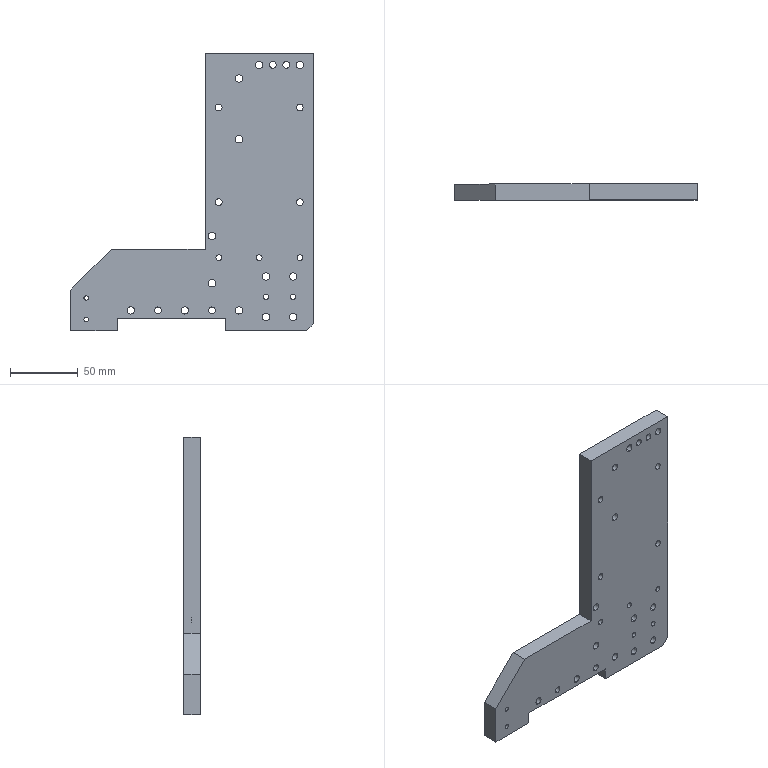Part | STEP file | PN_0006 | 1 solid | 117 faces | box 179.5 x 12 x 205 mm | volume 243420 mm3 | cylinder 86 | plane 27 | cone 4 | commonest cylinder face diameters 5.5 x26 10 x22 5 x16 4.2 x10 3.3 x4 4 x4